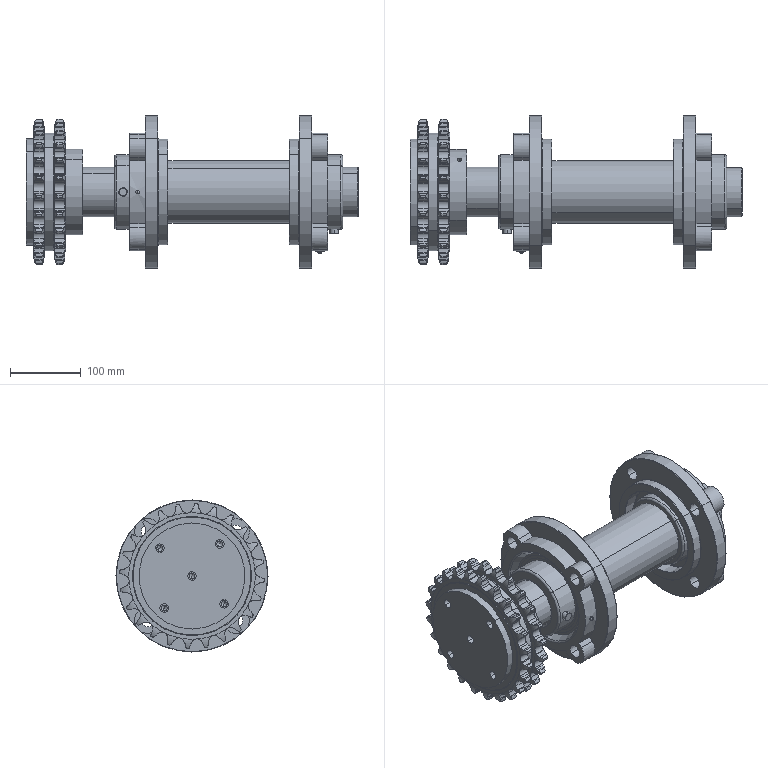Part | SolidWorks | 5 solids | 781 faces | box 469.5 x 215 x 215 mm | volume 5837825 mm3 | cylinder 430 | plane 161 | torus 156 | cone 34 | commonest cylinder face diameters 22.999 x100 41.467 x100 16.059 x62 206 x48 18.918 x16 12 x14